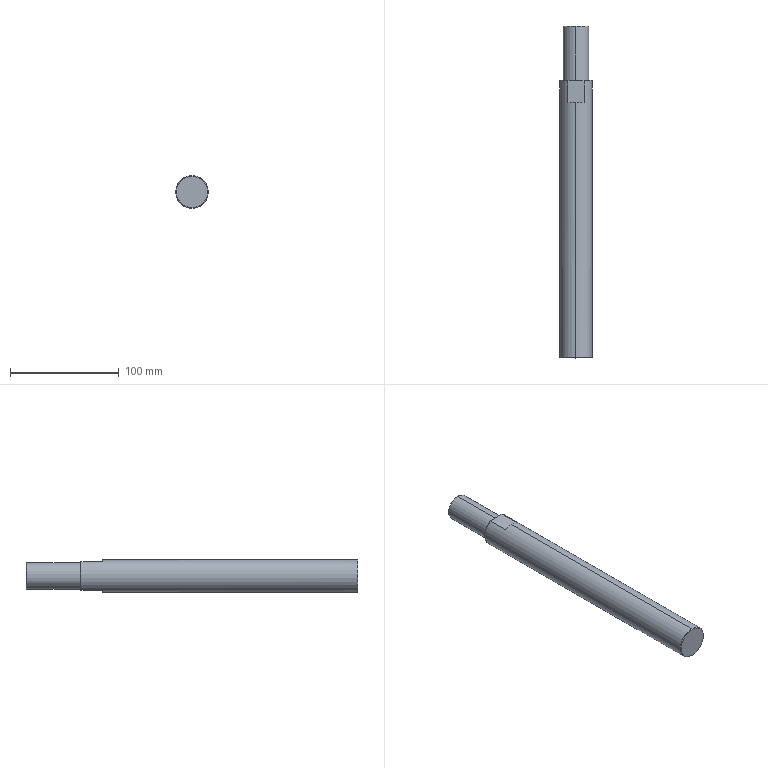Part | STEP file | 30 Plain Shaft | 1 solid | 17 faces | box 30 x 305 x 30 mm | volume 202030 mm3 | plane 7 | cone 6 | cylinder 4 | commonest cylinder face diameters 24 x2 30 x2
STEP:
#1=CARTESIAN_POINT('',(0.,0.,0.));
#2=DIRECTION('',(0.,0.,1.));
#3=DIRECTION('',(1.,0.,0.));
#4=AXIS2_PLACEMENT_3D('',#1,#2,#3);
#5=CARTESIAN_POINT('',(19295.293,8311.493,11.5));
#6=VERTEX_POINT('',#5);
#7=CARTESIAN_POINT('',(19295.293,8311.493,-11.5));
#8=VERTEX_POINT('',#7);
#9=CARTESIAN_POINT('',(19295.293,8311.493,0.));
#10=DIRECTION('',(0.,1.,0.));
#11=DIRECTION('',(0.,0.,1.));
#12=AXIS2_PLACEMENT_3D('',#9,#10,#11);
#13=CIRCLE('',#12,11.5);
#14=CARTESIAN_POINT('',(19295.293,8310.993,0.));
#15=DIRECTION('',(0.,-1.,0.));
#16=DIRECTION('',(0.,0.,-1.));
#17=AXIS2_PLACEMENT_3D('',#14,#15,#16);
#18=CONICAL_SURFACE('',#17,12.,0.7854);
#19=CARTESIAN_POINT('',(3.142,-0.5));
#20=DIRECTION('',(-1.,0.));
#21=VECTOR('',#20,1.);
#22=LINE('',#19,#21);
#23=(GEOMETRIC_REPRESENTATION_CONTEXT(2)PARAMETRIC_REPRESENTATION_CONTEXT()REPRESENTATION_CONTEXT('',''));
#24=DEFINITIONAL_REPRESENTATION('',(#22),#23);
#25=PCURVE('',#18,#24);
#26=CARTESIAN_POINT('',(19306.793,8311.493,0.));
#27=DIRECTION('',(0.,-1.,0.));
#28=DIRECTION('',(0.,0.,-1.));
#29=AXIS2_PLACEMENT_3D('',#26,#27,#28);
#30=PLANE('',#29);
#31=CARTESIAN_POINT('',(-11.5,-11.5));
#32=CARTESIAN_POINT('',(-11.5,8.419));
#33=CARTESIAN_POINT('',(5.75,-1.541));
#34=CARTESIAN_POINT('',(23.,-11.5));
#35=CARTESIAN_POINT('',(5.75,-21.459));
#36=CARTESIAN_POINT('',(-11.5,-31.419));
#37=CARTESIAN_POINT('',(-11.5,-11.5));
#38=(BOUNDED_CURVE()B_SPLINE_CURVE(2,(#31,#32,#33,#34,#35,#36,#37),.UNSPECIFIED.,.T.,.F.)B_SPLINE_CURVE_WITH_KNOTS((1,2,2,2,2,1),(-2.094,0.,2.094,4.189,6.283,8.378),.UNSPECIFIED.)CURVE()GEOMETRIC_REPRESENTATION_ITEM()RATIONAL_B_SPLINE_CURVE((1.,0.5,1.,0.5,1.,0.5,1.))REPRESENTATION_ITEM(''));
#39=(GEOMETRIC_REPRESENTATION_CONTEXT(2)PARAMETRIC_REPRESENTATION_CONTEXT()REPRESENTATION_CONTEXT('',''));
#40=DEFINITIONAL_REPRESENTATION('',(#38),#39);
#41=PCURVE('',#30,#40);
#42=SURFACE_CURVE('',#13,(#25,#41),.PCURVE_S1.);
#43=EDGE_CURVE('',#6,#8,#42,.T.);
#44=ORIENTED_EDGE('',*,*,#43,.F.);
#45=CARTESIAN_POINT('',(19295.293,8310.993,12.));
#46=VERTEX_POINT('',#45);
#47=CARTESIAN_POINT('',(19295.293,8310.993,12.));
#48=DIRECTION('',(0.,-0.7071,0.7071));
#49=VECTOR('',#48,1.);
#50=LINE('',#47,#49);
#51=CARTESIAN_POINT('',(3.142,0.));
#52=DIRECTION('',(0.,1.));
#53=VECTOR('',#52,1.);
#54=LINE('',#51,#53);
#55=(GEOMETRIC_REPRESENTATION_CONTEXT(2)PARAMETRIC_REPRESENTATION_CONTEXT()REPRESENTATION_CONTEXT('',''));
#56=DEFINITIONAL_REPRESENTATION('',(#54),#55);
#57=PCURVE('',#18,#56);
#58=CARTESIAN_POINT('',(19295.293,8310.993,0.));
#59=DIRECTION('',(0.,-1.,0.));
#60=DIRECTION('',(0.,0.,-1.));
#61=AXIS2_PLACEMENT_3D('',#58,#59,#60);
#62=CONICAL_SURFACE('',#61,12.,0.7854);
#63=CARTESIAN_POINT('',(3.142,0.));
#64=DIRECTION('',(0.,1.));
#65=VECTOR('',#64,1.);
#66=LINE('',#63,#65);
#67=(GEOMETRIC_REPRESENTATION_CONTEXT(2)PARAMETRIC_REPRESENTATION_CONTEXT()REPRESENTATION_CONTEXT('',''));
#68=DEFINITIONAL_REPRESENTATION('',(#66),#67);
#69=PCURVE('',#62,#68);
#70=SURFACE_CURVE('',#50,(#57,#69),.PCURVE_S1.);
#71=EDGE_CURVE('',#6,#46,#70,.T.);
#72=ORIENTED_EDGE('',*,*,#71,.T.);
#73=CARTESIAN_POINT('',(19295.293,8310.993,-12.));
#74=VERTEX_POINT('',#73);
#75=CARTESIAN_POINT('',(19295.293,8310.993,0.));
#76=DIRECTION('',(0.,1.,0.));
#77=DIRECTION('',(0.,0.,1.));
#78=AXIS2_PLACEMENT_3D('',#75,#76,#77);
#79=CIRCLE('',#78,12.);
#80=CARTESIAN_POINT('',(3.142,0.));
#81=DIRECTION('',(-1.,0.));
#82=VECTOR('',#81,1.);
#83=LINE('',#80,#82);
#84=(GEOMETRIC_REPRESENTATION_CONTEXT(2)PARAMETRIC_REPRESENTATION_CONTEXT()REPRESENTATION_CONTEXT('',''));
#85=DEFINITIONAL_REPRESENTATION('',(#83),#84);
#86=PCURVE('',#18,#85);
#87=CARTESIAN_POINT('',(19295.293,8358.766,0.));
#88=DIRECTION('',(0.,1.,0.));
#89=DIRECTION('',(0.,0.,1.));
#90=AXIS2_PLACEMENT_3D('',#87,#88,#89);
#91=CYLINDRICAL_SURFACE('',#90,12.);
#92=CARTESIAN_POINT('',(0.,-47.774));
#93=DIRECTION('',(1.,0.));
#94=VECTOR('',#93,1.);
#95=LINE('',#92,#94);
#96=(GEOMETRIC_REPRESENTATION_CONTEXT(2)PARAMETRIC_REPRESENTATION_CONTEXT()REPRESENTATION_CONTEXT('',''));
#97=DEFINITIONAL_REPRESENTATION('',(#95),#96);
#98=PCURVE('',#91,#97);
#99=SURFACE_CURVE('',#79,(#86,#98),.PCURVE_S1.);
#100=EDGE_CURVE('',#46,#74,#99,.T.);
#101=ORIENTED_EDGE('',*,*,#100,.T.);
#102=CARTESIAN_POINT('',(19295.293,8310.993,-12.));
#103=DIRECTION('',(0.,-0.7071,-0.7071));
#104=VECTOR('',#103,1.);
#105=LINE('',#102,#104);
#106=CARTESIAN_POINT('',(0.,0.));
#107=DIRECTION('',(0.,1.));
#108=VECTOR('',#107,1.);
#109=LINE('',#106,#108);
#110=(GEOMETRIC_REPRESENTATION_CONTEXT(2)PARAMETRIC_REPRESENTATION_CONTEXT()REPRESENTATION_CONTEXT('',''));
#111=DEFINITIONAL_REPRESENTATION('',(#109),#110);
#112=PCURVE('',#18,#111);
#113=CARTESIAN_POINT('',(6.283,0.));
#114=DIRECTION('',(0.,1.));
#115=VECTOR('',#114,1.);
#116=LINE('',#113,#115);
#117=(GEOMETRIC_REPRESENTATION_CONTEXT(2)PARAMETRIC_REPRESENTATION_CONTEXT()REPRESENTATION_CONTEXT('',''));
#118=DEFINITIONAL_REPRESENTATION('',(#116),#117);
#119=PCURVE('',#62,#118);
#120=SURFACE_CURVE('',#105,(#112,#119),.PCURVE_S1.);
#121=EDGE_CURVE('',#8,#74,#120,.T.);
#122=ORIENTED_EDGE('',*,*,#121,.F.);
#123=EDGE_LOOP('',(#44,#72,#101,#122));
#124=FACE_BOUND('',#123,.T.);
#125=ADVANCED_FACE('',(#124),#18,.T.);
#126=CARTESIAN_POINT('',(19295.293,8261.493,12.));
#127=VERTEX_POINT('',#126);
#128=CARTESIAN_POINT('',(19295.293,8261.493,-12.));
#129=VERTEX_POINT('',#128);
#130=CARTESIAN_POINT('',(19295.293,8261.493,0.));
#131=DIRECTION('',(0.,1.,0.));
#132=DIRECTION('',(0.,0.,1.));
#133=AXIS2_PLACEMENT_3D('',#130,#131,#132);
#134=CIRCLE('',#133,12.);
#135=CARTESIAN_POINT('',(0.,-97.274));
#136=DIRECTION('',(1.,0.));
#137=VECTOR('',#136,1.);
#138=LINE('',#135,#137);
#139=(GEOMETRIC_REPRESENTATION_CONTEXT(2)PARAMETRIC_REPRESENTATION_CONTEXT()REPRESENTATION_CONTEXT('',''));
#140=DEFINITIONAL_REPRESENTATION('',(#138),#139);
#141=PCURVE('',#91,#140);
#142=CARTESIAN_POINT('',(19309.793,8261.493,0.));
#143=DIRECTION('',(0.,-1.,0.));
#144=DIRECTION('',(0.,0.,-1.));
#145=AXIS2_PLACEMENT_3D('',#142,#143,#144);
#146=PLANE('',#145);
#147=CARTESIAN_POINT('',(-12.,-14.5));
#148=CARTESIAN_POINT('',(-12.,6.285));
#149=CARTESIAN_POINT('',(6.,-4.108));
#150=CARTESIAN_POINT('',(24.,-14.5));
#151=CARTESIAN_POINT('',(6.,-24.892));
#152=CARTESIAN_POINT('',(-12.,-35.285));
#153=CARTESIAN_POINT('',(-12.,-14.5));
#154=(BOUNDED_CURVE()B_SPLINE_CURVE(2,(#147,#148,#149,#150,#151,#152,#153),.UNSPECIFIED.,.T.,.F.)B_SPLINE_CURVE_WITH_KNOTS((1,2,2,2,2,1),(-2.094,0.,2.094,4.189,6.283,8.378),.UNSPECIFIED.)CURVE()GEOMETRIC_REPRESENTATION_ITEM()RATIONAL_B_SPLINE_CURVE((1.,0.5,1.,0.5,1.,0.5,1.))REPRESENTATION_ITEM(''));
#155=(GEOMETRIC_REPRESENTATION_CONTEXT(2)PARAMETRIC_REPRESENTATION_CONTEXT()REPRESENTATION_CONTEXT('',''));
#156=DEFINITIONAL_REPRESENTATION('',(#154),#155);
#157=PCURVE('',#146,#156);
#158=SURFACE_CURVE('',#134,(#141,#157),.PCURVE_S1.);
#159=EDGE_CURVE('',#127,#129,#158,.T.);
#160=ORIENTED_EDGE('',*,*,#159,.T.);
#161=CARTESIAN_POINT('',(19295.293,8358.766,-12.));
#162=DIRECTION('',(0.,1.,0.));
#163=VECTOR('',#162,1.);
#164=LINE('',#161,#163);
#165=CARTESIAN_POINT('',(3.142,0.));
#166=DIRECTION('',(0.,1.));
#167=VECTOR('',#166,1.);
#168=LINE('',#165,#167);
#169=(GEOMETRIC_REPRESENTATION_CONTEXT(2)PARAMETRIC_REPRESENTATION_CONTEXT()REPRESENTATION_CONTEXT('',''));
#170=DEFINITIONAL_REPRESENTATION('',(#168),#169);
#171=PCURVE('',#91,#170);
#172=CARTESIAN_POINT('',(19295.293,8358.766,0.));
#173=DIRECTION('',(0.,1.,0.));
#174=DIRECTION('',(0.,0.,1.));
#175=AXIS2_PLACEMENT_3D('',#172,#173,#174);
#176=CYLINDRICAL_SURFACE('',#175,12.);
#177=CARTESIAN_POINT('',(3.142,0.));
#178=DIRECTION('',(0.,1.));
#179=VECTOR('',#178,1.);
#180=LINE('',#177,#179);
#181=(GEOMETRIC_REPRESENTATION_CONTEXT(2)PARAMETRIC_REPRESENTATION_CONTEXT()REPRESENTATION_CONTEXT('',''));
#182=DEFINITIONAL_REPRESENTATION('',(#180),#181);
#183=PCURVE('',#176,#182);
#184=SURFACE_CURVE('',#164,(#171,#183),.PCURVE_S1.);
#185=EDGE_CURVE('',#129,#74,#184,.T.);
#186=ORIENTED_EDGE('',*,*,#185,.T.);
#187=ORIENTED_EDGE('',*,*,#100,.F.);
#188=CARTESIAN_POINT('',(19295.293,8358.766,12.));
#189=DIRECTION('',(0.,1.,0.));
#190=VECTOR('',#189,1.);
#191=LINE('',#188,#190);
#192=CARTESIAN_POINT('',(0.,0.));
#193=DIRECTION('',(0.,1.));
#194=VECTOR('',#193,1.);
#195=LINE('',#192,#194);
#196=(GEOMETRIC_REPRESENTATION_CONTEXT(2)PARAMETRIC_REPRESENTATION_CONTEXT()REPRESENTATION_CONTEXT('',''));
#197=DEFINITIONAL_REPRESENTATION('',(#195),#196);
#198=PCURVE('',#91,#197);
#199=CARTESIAN_POINT('',(6.283,0.));
#200=DIRECTION('',(0.,1.));
#201=VECTOR('',#200,1.);
#202=LINE('',#199,#201);
#203=(GEOMETRIC_REPRESENTATION_CONTEXT(2)PARAMETRIC_REPRESENTATION_CONTEXT()REPRESENTATION_CONTEXT('',''));
#204=DEFINITIONAL_REPRESENTATION('',(#202),#203);
#205=PCURVE('',#176,#204);
#206=SURFACE_CURVE('',#191,(#198,#205),.PCURVE_S1.);
#207=EDGE_CURVE('',#127,#46,#206,.T.);
#208=ORIENTED_EDGE('',*,*,#207,.F.);
#209=EDGE_LOOP('',(#160,#186,#187,#208));
#210=FACE_BOUND('',#209,.T.);
#211=ADVANCED_FACE('',(#210),#91,.T.);
#212=CARTESIAN_POINT('',(19295.293,8006.993,15.));
#213=VERTEX_POINT('',#212);
#214=CARTESIAN_POINT('',(19295.293,8006.993,-15.));
#215=VERTEX_POINT('',#214);
#216=CARTESIAN_POINT('',(19295.293,8006.993,0.));
#217=DIRECTION('',(0.,1.,0.));
#218=DIRECTION('',(0.,0.,1.));
#219=AXIS2_PLACEMENT_3D('',#216,#217,#218);
#220=CIRCLE('',#219,15.);
#221=CARTESIAN_POINT('',(19295.293,8358.766,0.));
#222=DIRECTION('',(0.,1.,0.));
#223=DIRECTION('',(0.,0.,1.));
#224=AXIS2_PLACEMENT_3D('',#221,#222,#223);
#225=CYLINDRICAL_SURFACE('',#224,15.);
#226=CARTESIAN_POINT('',(0.,-351.774));
#227=DIRECTION('',(1.,0.));
#228=VECTOR('',#227,1.);
#229=LINE('',#226,#228);
#230=(GEOMETRIC_REPRESENTATION_CONTEXT(2)PARAMETRIC_REPRESENTATION_CONTEXT()REPRESENTATION_CONTEXT('',''));
#231=DEFINITIONAL_REPRESENTATION('',(#229),#230);
#232=PCURVE('',#225,#231);
#233=CARTESIAN_POINT('',(19295.293,8006.493,0.));
#234=DIRECTION('',(0.,1.,0.));
#235=DIRECTION('',(0.,0.,1.));
#236=AXIS2_PLACEMENT_3D('',#233,#234,#235);
#237=CONICAL_SURFACE('',#236,14.5,0.7854);
#238=CARTESIAN_POINT('',(0.,0.5));
#239=DIRECTION('',(1.,0.));
#240=VECTOR('',#239,1.);
#241=LINE('',#238,#240);
#242=(GEOMETRIC_REPRESENTATION_CONTEXT(2)PARAMETRIC_REPRESENTATION_CONTEXT()REPRESENTATION_CONTEXT('',''));
#243=DEFINITIONAL_REPRESENTATION('',(#241),#242);
#244=PCURVE('',#237,#243);
#245=SURFACE_CURVE('',#220,(#232,#244),.PCURVE_S1.);
#246=EDGE_CURVE('',#213,#215,#245,.T.);
#247=ORIENTED_EDGE('',*,*,#246,.T.);
#248=CARTESIAN_POINT('',(19295.293,8241.493,-15.));
#249=VERTEX_POINT('',#248);
#250=CARTESIAN_POINT('',(19295.293,8358.766,-15.));
#251=DIRECTION('',(0.,1.,0.));
#252=VECTOR('',#251,1.);
#253=LINE('',#250,#252);
#254=CARTESIAN_POINT('',(3.142,0.));
#255=DIRECTION('',(0.,1.));
#256=VECTOR('',#255,1.);
#257=LINE('',#254,#256);
#258=(GEOMETRIC_REPRESENTATION_CONTEXT(2)PARAMETRIC_REPRESENTATION_CONTEXT()REPRESENTATION_CONTEXT('',''));
#259=DEFINITIONAL_REPRESENTATION('',(#257),#258);
#260=PCURVE('',#225,#259);
#261=CARTESIAN_POINT('',(19295.293,8358.766,0.));
#262=DIRECTION('',(0.,1.,0.));
#263=DIRECTION('',(0.,0.,1.));
#264=AXIS2_PLACEMENT_3D('',#261,#262,#263);
#265=CYLINDRICAL_SURFACE('',#264,15.);
#266=CARTESIAN_POINT('',(3.142,0.));
#267=DIRECTION('',(0.,1.));
#268=VECTOR('',#267,1.);
#269=LINE('',#266,#268);
#270=(GEOMETRIC_REPRESENTATION_CONTEXT(2)PARAMETRIC_REPRESENTATION_CONTEXT()REPRESENTATION_CONTEXT('',''));
#271=DEFINITIONAL_REPRESENTATION('',(#269),#270);
#272=PCURVE('',#265,#271);
#273=SURFACE_CURVE('',#253,(#260,#272),.PCURVE_S1.);
#274=EDGE_CURVE('',#215,#249,#273,.T.);
#275=ORIENTED_EDGE('',*,*,#274,.T.);
#276=CARTESIAN_POINT('',(19302.777,8241.493,-13.));
#277=VERTEX_POINT('',#276);
#278=CARTESIAN_POINT('',(19295.293,8241.493,0.));
#279=DIRECTION('',(0.,1.,0.));
#280=DIRECTION('',(0.,0.,1.));
#281=AXIS2_PLACEMENT_3D('',#278,#279,#280);
#282=CIRCLE('',#281,15.);
#283=CARTESIAN_POINT('',(0.,-117.274));
#284=DIRECTION('',(1.,0.));
#285=VECTOR('',#284,1.);
#286=LINE('',#283,#285);
#287=(GEOMETRIC_REPRESENTATION_CONTEXT(2)PARAMETRIC_REPRESENTATION_CONTEXT()REPRESENTATION_CONTEXT('',''));
#288=DEFINITIONAL_REPRESENTATION('',(#286),#287);
#289=PCURVE('',#225,#288);
#290=CARTESIAN_POINT('',(0.,8241.493,0.));
#291=DIRECTION('',(0.,1.,0.));
#292=DIRECTION('',(0.,0.,1.));
#293=AXIS2_PLACEMENT_3D('',#290,#291,#292);
#294=PLANE('',#293);
#295=CARTESIAN_POINT('',(0.,19295.293));
#296=DIRECTION('',(1.,0.));
#297=AXIS2_PLACEMENT_2D('',#295,#296);
#298=CIRCLE('',#297,15.);
#299=(GEOMETRIC_REPRESENTATION_CONTEXT(2)PARAMETRIC_REPRESENTATION_CONTEXT()REPRESENTATION_CONTEXT('',''));
#300=DEFINITIONAL_REPRESENTATION('',(#298),#299);
#301=PCURVE('',#294,#300);
#302=SURFACE_CURVE('',#282,(#289,#301),.PCURVE_S1.);
#303=EDGE_CURVE('',#277,#249,#302,.T.);
#304=ORIENTED_EDGE('',*,*,#303,.F.);
#305=CARTESIAN_POINT('',(19302.777,8260.993,-13.));
#306=VERTEX_POINT('',#305);
#307=CARTESIAN_POINT('',(19302.777,8358.766,-13.));
#308=DIRECTION('',(0.,1.,0.));
#309=VECTOR('',#308,1.);
#310=LINE('',#307,#309);
#311=CARTESIAN_POINT('',(2.619,0.));
#312=DIRECTION('',(0.,1.));
#313=VECTOR('',#312,1.);
#314=LINE('',#311,#313);
#315=(GEOMETRIC_REPRESENTATION_CONTEXT(2)PARAMETRIC_REPRESENTATION_CONTEXT()REPRESENTATION_CONTEXT('',''));
#316=DEFINITIONAL_REPRESENTATION('',(#314),#315);
#317=PCURVE('',#225,#316);
#318=CARTESIAN_POINT('',(19265.494,8241.493,-13.));
#319=DIRECTION('',(0.,0.,1.));
#320=DIRECTION('',(1.,0.,0.));
#321=AXIS2_PLACEMENT_3D('',#318,#319,#320);
#322=PLANE('',#321);
#323=CARTESIAN_POINT('',(37.282,117.274));
#324=DIRECTION('',(0.,1.));
#325=VECTOR('',#324,1.);
#326=LINE('',#323,#325);
#327=(GEOMETRIC_REPRESENTATION_CONTEXT(2)PARAMETRIC_REPRESENTATION_CONTEXT()REPRESENTATION_CONTEXT('',''));
#328=DEFINITIONAL_REPRESENTATION('',(#326),#327);
#329=PCURVE('',#322,#328);
#330=SURFACE_CURVE('',#310,(#317,#329),.PCURVE_S1.);
#331=EDGE_CURVE('',#277,#306,#330,.T.);
#332=ORIENTED_EDGE('',*,*,#331,.T.);
#333=CARTESIAN_POINT('',(19302.777,8260.993,13.));
#334=VERTEX_POINT('',#333);
#335=CARTESIAN_POINT('',(19295.293,8260.993,0.));
#336=DIRECTION('',(0.,1.,0.));
#337=DIRECTION('',(0.,0.,1.));
#338=AXIS2_PLACEMENT_3D('',#335,#336,#337);
#339=CIRCLE('',#338,15.);
#340=CARTESIAN_POINT('',(0.,-97.774));
#341=DIRECTION('',(1.,0.));
#342=VECTOR('',#341,1.);
#343=LINE('',#340,#342);
#344=(GEOMETRIC_REPRESENTATION_CONTEXT(2)PARAMETRIC_REPRESENTATION_CONTEXT()REPRESENTATION_CONTEXT('',''));
#345=DEFINITIONAL_REPRESENTATION('',(#343),#344);
#346=PCURVE('',#225,#345);
#347=CARTESIAN_POINT('',(19295.293,8260.993,0.));
#348=DIRECTION('',(0.,-1.,0.));
#349=DIRECTION('',(0.,0.,-1.));
#350=AXIS2_PLACEMENT_3D('',#347,#348,#349);
#351=CONICAL_SURFACE('',#350,15.,0.7854);
#352=CARTESIAN_POINT('',(3.142,0.));
#353=DIRECTION('',(-1.,0.));
#354=VECTOR('',#353,1.);
#355=LINE('',#352,#354);
#356=(GEOMETRIC_REPRESENTATION_CONTEXT(2)PARAMETRIC_REPRESENTATION_CONTEXT()REPRESENTATION_CONTEXT('',''));
#357=DEFINITIONAL_REPRESENTATION('',(#355),#356);
#358=PCURVE('',#351,#357);
#359=SURFACE_CURVE('',#339,(#346,#358),.PCURVE_S1.);
#360=EDGE_CURVE('',#334,#306,#359,.T.);
#361=ORIENTED_EDGE('',*,*,#360,.F.);
#362=CARTESIAN_POINT('',(19302.777,8241.493,13.));
#363=VERTEX_POINT('',#362);
#364=CARTESIAN_POINT('',(19302.777,8358.766,13.));
#365=DIRECTION('',(0.,-1.,0.));
#366=VECTOR('',#365,1.);
#367=LINE('',#364,#366);
#368=CARTESIAN_POINT('',(0.5223,0.));
#369=DIRECTION('',(0.,-1.));
#370=VECTOR('',#369,1.);
#371=LINE('',#368,#370);
#372=(GEOMETRIC_REPRESENTATION_CONTEXT(2)PARAMETRIC_REPRESENTATION_CONTEXT()REPRESENTATION_CONTEXT('',''));
#373=DEFINITIONAL_REPRESENTATION('',(#371),#372);
#374=PCURVE('',#225,#373);
#375=CARTESIAN_POINT('',(19286.893,8241.493,13.));
#376=DIRECTION('',(0.,0.,-1.));
#377=DIRECTION('',(-1.,0.,0.));
#378=AXIS2_PLACEMENT_3D('',#375,#376,#377);
#379=PLANE('',#378);
#380=CARTESIAN_POINT('',(-15.884,117.274));
#381=DIRECTION('',(0.,-1.));
#382=VECTOR('',#381,1.);
#383=LINE('',#380,#382);
#384=(GEOMETRIC_REPRESENTATION_CONTEXT(2)PARAMETRIC_REPRESENTATION_CONTEXT()REPRESENTATION_CONTEXT('',''));
#385=DEFINITIONAL_REPRESENTATION('',(#383),#384);
#386=PCURVE('',#379,#385);
#387=SURFACE_CURVE('',#367,(#374,#386),.PCURVE_S1.);
#388=EDGE_CURVE('',#334,#363,#387,.T.);
#389=ORIENTED_EDGE('',*,*,#388,.T.);
#390=CARTESIAN_POINT('',(19295.293,8241.493,15.));
#391=VERTEX_POINT('',#390);
#392=CARTESIAN_POINT('',(19295.293,8241.493,0.));
#393=DIRECTION('',(0.,-1.,0.));
#394=DIRECTION('',(0.,0.,-1.));
#395=AXIS2_PLACEMENT_3D('',#392,#393,#394);
#396=CIRCLE('',#395,15.);
#397=CARTESIAN_POINT('',(3.142,-117.274));
#398=DIRECTION('',(-1.,0.));
#399=VECTOR('',#398,1.);
#400=LINE('',#397,#399);
#401=(GEOMETRIC_REPRESENTATION_CONTEXT(2)PARAMETRIC_REPRESENTATION_CONTEXT()REPRESENTATION_CONTEXT('',''));
#402=DEFINITIONAL_REPRESENTATION('',(#400),#401);
#403=PCURVE('',#225,#402);
#404=CARTESIAN_POINT('',(0.,8241.493,0.));
#405=DIRECTION('',(0.,-1.,0.));
#406=DIRECTION('',(0.,0.,-1.));
#407=AXIS2_PLACEMENT_3D('',#404,#405,#406);
#408=PLANE('',#407);
#409=CARTESIAN_POINT('',(0.,19295.293));
#410=DIRECTION('',(1.,0.));
#411=AXIS2_PLACEMENT_2D('',#409,#410);
#412=CIRCLE('',#411,15.);
#413=(GEOMETRIC_REPRESENTATION_CONTEXT(2)PARAMETRIC_REPRESENTATION_CONTEXT()REPRESENTATION_CONTEXT('',''));
#414=DEFINITIONAL_REPRESENTATION('',(#412),#413);
#415=PCURVE('',#408,#414);
#416=SURFACE_CURVE('',#396,(#403,#415),.PCURVE_S1.);
#417=EDGE_CURVE('',#363,#391,#416,.T.);
#418=ORIENTED_EDGE('',*,*,#417,.T.);
#419=CARTESIAN_POINT('',(19295.293,8358.766,15.));
#420=DIRECTION('',(0.,1.,0.));
#421=VECTOR('',#420,1.);
#422=LINE('',#419,#421);
#423=CARTESIAN_POINT('',(0.,0.));
#424=DIRECTION('',(0.,1.));
#425=VECTOR('',#424,1.);
#426=LINE('',#423,#425);
#427=(GEOMETRIC_REPRESENTATION_CONTEXT(2)PARAMETRIC_REPRESENTATION_CONTEXT()REPRESENTATION_CONTEXT('',''));
#428=DEFINITIONAL_REPRESENTATION('',(#426),#427);
#429=PCURVE('',#225,#428);
#430=CARTESIAN_POINT('',(6.283,0.));
#431=DIRECTION('',(0.,1.));
#432=VECTOR('',#431,1.);
#433=LINE('',#430,#432);
#434=(GEOMETRIC_REPRESENTATION_CONTEXT(2)PARAMETRIC_REPRESENTATION_CONTEXT()REPRESENTATION_CONTEXT('',''));
#435=DEFINITIONAL_REPRESENTATION('',(#433),#434);
#436=PCURVE('',#265,#435);
#437=SURFACE_CURVE('',#422,(#429,#436),.PCURVE_S1.);
#438=EDGE_CURVE('',#213,#391,#437,.T.);
#439=ORIENTED_EDGE('',*,*,#438,.F.);
#440=EDGE_LOOP('',(#247,#275,#304,#332,#361,#389,#418,#439));
#441=FACE_BOUND('',#440,.T.);
#442=ADVANCED_FACE('',(#441),#225,.T.);
#443=CARTESIAN_POINT('',(19295.293,8006.493,14.5));
#444=VERTEX_POINT('',#443);
#445=CARTESIAN_POINT('',(19295.293,8006.493,-14.5));
#446=VERTEX_POINT('',#445);
#447=CARTESIAN_POINT('',(19295.293,8006.493,0.));
#448=DIRECTION('',(0.,1.,0.));
#449=DIRECTION('',(0.,0.,1.));
#450=AXIS2_PLACEMENT_3D('',#447,#448,#449);
#451=CIRCLE('',#450,14.5);
#452=CARTESIAN_POINT('',(0.,0.));
#453=DIRECTION('',(1.,0.));
#454=VECTOR('',#453,1.);
#455=LINE('',#452,#454);
#456=(GEOMETRIC_REPRESENTATION_CONTEXT(2)PARAMETRIC_REPRESENTATION_CONTEXT()REPRESENTATION_CONTEXT('',''));
#457=DEFINITIONAL_REPRESENTATION('',(#455),#456);
#458=PCURVE('',#237,#457);
#459=CARTESIAN_POINT('',(19307.293,8006.493,0.));
#460=DIRECTION('',(0.,1.,0.));
#461=DIRECTION('',(0.,0.,1.));
#462=AXIS2_PLACEMENT_3D('',#459,#460,#461);
#463=PLANE('',#462);
#464=CARTESIAN_POINT('',(0.,-12.));
#465=DIRECTION('',(1.,0.));
#466=AXIS2_PLACEMENT_2D('',#464,#465);
#467=CIRCLE('',#466,14.5);
#468=(GEOMETRIC_REPRESENTATION_CONTEXT(2)PARAMETRIC_REPRESENTATION_CONTEXT()REPRESENTATION_CONTEXT('',''));
#469=DEFINITIONAL_REPRESENTATION('',(#467),#468);
#470=PCURVE('',#463,#469);
#471=SURFACE_CURVE('',#451,(#458,#470),.PCURVE_S1.);
#472=EDGE_CURVE('',#444,#446,#471,.T.);
#473=ORIENTED_EDGE('',*,*,#472,.T.);
#474=CARTESIAN_POINT('',(19295.293,8006.493,-14.5));
#475=DIRECTION('',(0.,0.7071,-0.7071));
#476=VECTOR('',#475,1.);
#477=LINE('',#474,#476);
#478=CARTESIAN_POINT('',(3.142,0.));
#479=DIRECTION('',(0.,1.));
#480=VECTOR('',#479,1.);
#481=LINE('',#478,#480);
#482=(GEOMETRIC_REPRESENTATION_CONTEXT(2)PARAMETRIC_REPRESENTATION_CONTEXT()REPRESENTATION_CONTEXT('',''));
#483=DEFINITIONAL_REPRESENTATION('',(#481),#482);
#484=PCURVE('',#237,#483);
#485=CARTESIAN_POINT('',(19295.293,8006.493,0.));
#486=DIRECTION('',(0.,1.,0.));
#487=DIRECTION('',(0.,0.,1.));
#488=AXIS2_PLACEMENT_3D('',#485,#486,#487);
#489=CONICAL_SURFACE('',#488,14.5,0.7854);
#490=CARTESIAN_POINT('',(3.142,0.));
#491=DIRECTION('',(0.,1.));
#492=VECTOR('',#491,1.);
#493=LINE('',#490,#492);
#494=(GEOMETRIC_REPRESENTATION_CONTEXT(2)PARAMETRIC_REPRESENTATION_CONTEXT()REPRESENTATION_CONTEXT('',''));
#495=DEFINITIONAL_REPRESENTATION('',(#493),#494);
#496=PCURVE('',#489,#495);
#497=SURFACE_CURVE('',#477,(#484,#496),.PCURVE_S1.);
#498=EDGE_CURVE('',#446,#215,#497,.T.);
#499=ORIENTED_EDGE('',*,*,#498,.T.);
#500=ORIENTED_EDGE('',*,*,#246,.F.);
#501=CARTESIAN_POINT('',(19295.293,8006.493,14.5));
#502=DIRECTION('',(0.,0.7071,0.7071));
#503=VECTOR('',#502,1.);
#504=LINE('',#501,#503);
#505=CARTESIAN_POINT('',(0.,0.));
#506=DIRECTION('',(0.,1.));
#507=VECTOR('',#506,1.);
#508=LINE('',#505,#507);
#509=(GEOMETRIC_REPRESENTATION_CONTEXT(2)PARAMETRIC_REPRESENTATION_CONTEXT()REPRESENTATION_CONTEXT('',''));
#510=DEFINITIONAL_REPRESENTATION('',(#508),#509);
#511=PCURVE('',#237,#510);
#512=CARTESIAN_POINT('',(6.283,0.));
#513=DIRECTION('',(0.,1.));
#514=VECTOR('',#513,1.);
#515=LINE('',#512,#514);
#516=(GEOMETRIC_REPRESENTATION_CONTEXT(2)PARAMETRIC_REPRESENTATION_CONTEXT()REPRESENTATION_CONTEXT('',''));
#517=DEFINITIONAL_REPRESENTATION('',(#515),#516);
#518=PCURVE('',#489,#517);
#519=SURFACE_CURVE('',#504,(#511,#518),.PCURVE_S1.);
#520=EDGE_CURVE('',#444,#213,#519,.T.);
#521=ORIENTED_EDGE('',*,*,#520,.F.);
#522=EDGE_LOOP('',(#473,#499,#500,#521));
#523=FACE_BOUND('',#522,.T.);
#524=ADVANCED_FACE('',(#523),#237,.T.);
#525=CARTESIAN_POINT('',(19287.81,8260.993,-13.));
#526=VERTEX_POINT('',#525);
#527=CARTESIAN_POINT('',(19287.81,8260.993,13.));
#528=VERTEX_POINT('',#527);
#529=CARTESIAN_POINT('',(19295.293,8260.993,0.));
#530=DIRECTION('',(0.,1.,0.));
#531=DIRECTION('',(0.,0.,1.));
#532=AXIS2_PLACEMENT_3D('',#529,#530,#531);
#533=CIRCLE('',#532,15.);
#534=CARTESIAN_POINT('',(19295.293,8260.993,0.));
#535=DIRECTION('',(0.,-1.,0.));
#536=DIRECTION('',(0.,0.,-1.));
#537=AXIS2_PLACEMENT_3D('',#534,#535,#536);
#538=CONICAL_SURFACE('',#537,15.,0.7854);
#539=CARTESIAN_POINT('',(9.425,0.));
#540=DIRECTION('',(-1.,0.));
#541=VECTOR('',#540,1.);
#542=LINE('',#539,#541);
#543=(GEOMETRIC_REPRESENTATION_CONTEXT(2)PARAMETRIC_REPRESENTATION_CONTEXT()REPRESENTATION_CONTEXT('',''));
#544=DEFINITIONAL_REPRESENTATION('',(#542),#543);
#545=PCURVE('',#538,#544);
#546=CARTESIAN_POINT('',(0.,-97.774));
#547=DIRECTION('',(1.,0.));
#548=VECTOR('',#547,1.);
#549=LINE('',#546,#548);
#550=(GEOMETRIC_REPRESENTATION_CONTEXT(2)PARAMETRIC_REPRESENTATION_CONTEXT()REPRESENTATION_CONTEXT('',''));
#551=DEFINITIONAL_REPRESENTATION('',(#549),#550);
#552=PCURVE('',#265,#551);
#553=SURFACE_CURVE('',#533,(#545,#552),.PCURVE_S1.);
#554=EDGE_CURVE('',#526,#528,#553,.T.);
#555=ORIENTED_EDGE('',*,*,#554,.T.);
#556=CARTESIAN_POINT('',(19288.871,8261.493,13.));
#557=VERTEX_POINT('',#556);
#558=CARTESIAN_POINT('',(19287.81,8260.993,13.));
#559=CARTESIAN_POINT('',(19288.159,8261.167,13.));
#560=CARTESIAN_POINT('',(19288.512,8261.334,13.));
#561=CARTESIAN_POINT('',(19288.871,8261.493,13.));
#562=B_SPLINE_CURVE_WITH_KNOTS('',3,(#558,#559,#560,#561),.UNSPECIFIED.,.F.,.F.,(4,4),(0.0186,0.01977),.PIECEWISE_BEZIER_KNOTS.);
#563=CARTESIAN_POINT('',(3.664,0.));
#564=CARTESIAN_POINT('',(3.663,-0.007919));
#565=CARTESIAN_POINT('',(3.661,-0.02373));
#566=CARTESIAN_POINT('',(3.658,-0.04735));
#567=CARTESIAN_POINT('',(3.656,-0.07089));
#568=CARTESIAN_POINT('',(3.653,-0.09433));
#569=CARTESIAN_POINT('',(3.65,-0.1177));
#570=CARTESIAN_POINT('',(3.647,-0.141));
#571=CARTESIAN_POINT('',(3.644,-0.1641));
#572=CARTESIAN_POINT('',(3.642,-0.1872));
#573=CARTESIAN_POINT('',(3.639,-0.2102));
#574=CARTESIAN_POINT('',(3.636,-0.2331));
#575=CARTESIAN_POINT('',(3.633,-0.2559));
#576=CARTESIAN_POINT('',(3.63,-0.2786));
#577=CARTESIAN_POINT('',(3.627,-0.3011));
#578=CARTESIAN_POINT('',(3.624,-0.3236));
#579=CARTESIAN_POINT('',(3.621,-0.346));
#580=CARTESIAN_POINT('',(3.618,-0.3683));
#581=CARTESIAN_POINT('',(3.615,-0.3905));
#582=CARTESIAN_POINT('',(3.612,-0.4126));
#583=CARTESIAN_POINT('',(3.609,-0.4346));
#584=CARTESIAN_POINT('',(3.606,-0.4565));
#585=CARTESIAN_POINT('',(3.603,-0.4783));
#586=CARTESIAN_POINT('',(3.601,-0.4928));
#587=CARTESIAN_POINT('',(3.6,-0.5));
#588=B_SPLINE_CURVE_WITH_KNOTS('',3,(#563,#564,#565,#566,#567,#568,#569,#570,#571,#572,#573,#574,#575,#576,#577,#578,#579,#580,#581,#582,#583,#584,#585,#586,#587),.UNSPECIFIED.,.F.,.F.,(4,1,1,1,1,1,1,1,1,1,1,1,1,1,1,1,1,1,1,1,1,1,4),(0.0186,0.01865,0.01871,0.01876,0.01881,0.01887,0.01892,0.01897,0.01903,0.01908,0.01913,0.01919,0.01924,0.01929,0.01935,0.0194,0.01945,0.01951,0.01956,0.01961,0.01967,0.01972,0.01977),.QUASI_UNIFORM_KNOTS.);
#589=(GEOMETRIC_REPRESENTATION_CONTEXT(2)PARAMETRIC_REPRESENTATION_CONTEXT()REPRESENTATION_CONTEXT('',''));
#590=DEFINITIONAL_REPRESENTATION('',(#588),#589);
#591=PCURVE('',#538,#590);
#592=CARTESIAN_POINT('',(-0.917,19.5));
#593=CARTESIAN_POINT('',(-1.266,19.674));
#594=CARTESIAN_POINT('',(-1.62,19.841));
#595=CARTESIAN_POINT('',(-1.978,20.));
#596=B_SPLINE_CURVE_WITH_KNOTS('',3,(#592,#593,#594,#595),.UNSPECIFIED.,.F.,.F.,(4,4),(0.0186,0.01977),.PIECEWISE_BEZIER_KNOTS.);
#597=(GEOMETRIC_REPRESENTATION_CONTEXT(2)PARAMETRIC_REPRESENTATION_CONTEXT()REPRESENTATION_CONTEXT('',''));
#598=DEFINITIONAL_REPRESENTATION('',(#596),#597);
#599=PCURVE('',#379,#598);
#600=SURFACE_CURVE('',#562,(#591,#599),.PCURVE_S1.);
#601=EDGE_CURVE('',#528,#557,#600,.T.);
#602=ORIENTED_EDGE('',*,*,#601,.T.);
#603=CARTESIAN_POINT('',(19288.871,8261.493,-13.));
#604=VERTEX_POINT('',#603);
#605=CARTESIAN_POINT('',(19295.293,8261.493,0.));
#606=DIRECTION('',(0.,1.,0.));
#607=DIRECTION('',(0.,0.,1.));
#608=AXIS2_PLACEMENT_3D('',#605,#606,#607);
#609=CIRCLE('',#608,14.5);
#610=CARTESIAN_POINT('',(9.425,-0.5));
#611=DIRECTION('',(-1.,0.));
#612=VECTOR('',#611,1.);
#613=LINE('',#610,#612);
#614=(GEOMETRIC_REPRESENTATION_CONTEXT(2)PARAMETRIC_REPRESENTATION_CONTEXT()REPRESENTATION_CONTEXT('',''));
#615=DEFINITIONAL_REPRESENTATION('',(#613),#614);
#616=PCURVE('',#538,#615);
#617=CARTESIAN_POINT('',(-14.5,-14.5));
#618=CARTESIAN_POINT('',(-14.5,10.615));
#619=CARTESIAN_POINT('',(7.25,-1.943));
#620=CARTESIAN_POINT('',(29.,-14.5));
#621=CARTESIAN_POINT('',(7.25,-27.057));
#622=CARTESIAN_POINT('',(-14.5,-39.615));
#623=CARTESIAN_POINT('',(-14.5,-14.5));
#624=(BOUNDED_CURVE()B_SPLINE_CURVE(2,(#617,#618,#619,#620,#621,#622,#623),.UNSPECIFIED.,.T.,.F.)B_SPLINE_CURVE_WITH_KNOTS((1,2,2,2,2,1),(-2.094,0.,2.094,4.189,6.283,8.378),.UNSPECIFIED.)CURVE()GEOMETRIC_REPRESENTATION_ITEM()RATIONAL_B_SPLINE_CURVE((1.,0.5,1.,0.5,1.,0.5,1.))REPRESENTATION_ITEM(''));
#625=(GEOMETRIC_REPRESENTATION_CONTEXT(2)PARAMETRIC_REPRESENTATION_CONTEXT()REPRESENTATION_CONTEXT('',''));
#626=DEFINITIONAL_REPRESENTATION('',(#624),#625);
#627=PCURVE('',#146,#626);
#628=SURFACE_CURVE('',#609,(#616,#627),.PCURVE_S1.);
#629=EDGE_CURVE('',#604,#557,#628,.T.);
#630=ORIENTED_EDGE('',*,*,#629,.F.);
#631=CARTESIAN_POINT('',(19288.871,8261.493,-13.));
#632=CARTESIAN_POINT('',(19288.512,8261.334,-13.));
#633=CARTESIAN_POINT('',(19288.159,8261.167,-13.));
#634=CARTESIAN_POINT('',(19287.81,8260.993,-13.));
#635=B_SPLINE_CURVE_WITH_KNOTS('',3,(#631,#632,#633,#634),.UNSPECIFIED.,.F.,.F.,(4,4),(0.04363,0.04481),.PIECEWISE_BEZIER_KNOTS.);
#636=CARTESIAN_POINT('',(5.824,-0.5));
#637=CARTESIAN_POINT('',(5.823,-0.4928));
#638=CARTESIAN_POINT('',(5.821,-0.4783));
#639=CARTESIAN_POINT('',(5.818,-0.4565));
#640=CARTESIAN_POINT('',(5.815,-0.4346));
#641=CARTESIAN_POINT('',(5.812,-0.4126));
#642=CARTESIAN_POINT('',(5.809,-0.3905));
#643=CARTESIAN_POINT('',(5.806,-0.3683));
#644=CARTESIAN_POINT('',(5.803,-0.346));
#645=CARTESIAN_POINT('',(5.801,-0.3236));
#646=CARTESIAN_POINT('',(5.798,-0.3011));
#647=CARTESIAN_POINT('',(5.795,-0.2785));
#648=CARTESIAN_POINT('',(5.792,-0.2558));
#649=CARTESIAN_POINT('',(5.789,-0.233));
#650=CARTESIAN_POINT('',(5.786,-0.2101));
#651=CARTESIAN_POINT('',(5.783,-0.1872));
#652=CARTESIAN_POINT('',(5.78,-0.1641));
#653=CARTESIAN_POINT('',(5.778,-0.1409));
#654=CARTESIAN_POINT('',(5.775,-0.1177));
#655=CARTESIAN_POINT('',(5.772,-0.09431));
#656=CARTESIAN_POINT('',(5.769,-0.07087));
#657=CARTESIAN_POINT('',(5.766,-0.04734));
#658=CARTESIAN_POINT('',(5.764,-0.02372));
#659=CARTESIAN_POINT('',(5.762,-0.007917));
#660=CARTESIAN_POINT('',(5.761,0.));
#661=B_SPLINE_CURVE_WITH_KNOTS('',3,(#636,#637,#638,#639,#640,#641,#642,#643,#644,#645,#646,#647,#648,#649,#650,#651,#652,#653,#654,#655,#656,#657,#658,#659,#660),.UNSPECIFIED.,.F.,.F.,(4,1,1,1,1,1,1,1,1,1,1,1,1,1,1,1,1,1,1,1,1,1,4),(0.04363,0.04369,0.04374,0.04379,0.04385,0.0439,0.04395,0.04401,0.04406,0.04411,0.04417,0.04422,0.04428,0.04433,0.04438,0.04444,0.04449,0.04454,0.0446,0.04465,0.0447,0.04476,0.04481),.QUASI_UNIFORM_KNOTS.);
#662=(GEOMETRIC_REPRESENTATION_CONTEXT(2)PARAMETRIC_REPRESENTATION_CONTEXT()REPRESENTATION_CONTEXT('',''));
#663=DEFINITIONAL_REPRESENTATION('',(#661),#662);
#664=PCURVE('',#538,#663);
#665=CARTESIAN_POINT('',(23.376,20.));
#666=CARTESIAN_POINT('',(23.018,19.841));
#667=CARTESIAN_POINT('',(22.665,19.674));
#668=CARTESIAN_POINT('',(22.316,19.5));
#669=B_SPLINE_CURVE_WITH_KNOTS('',3,(#665,#666,#667,#668),.UNSPECIFIED.,.F.,.F.,(4,4),(0.04363,0.04481),.PIECEWISE_BEZIER_KNOTS.);
#670=(GEOMETRIC_REPRESENTATION_CONTEXT(2)PARAMETRIC_REPRESENTATION_CONTEXT()REPRESENTATION_CONTEXT('',''));
#671=DEFINITIONAL_REPRESENTATION('',(#669),#670);
#672=PCURVE('',#322,#671);
#673=SURFACE_CURVE('',#635,(#664,#672),.PCURVE_S1.);
#674=EDGE_CURVE('',#604,#526,#673,.T.);
#675=ORIENTED_EDGE('',*,*,#674,.T.);
#676=EDGE_LOOP('',(#555,#602,#630,#675));
#677=FACE_BOUND('',#676,.T.);
#678=ADVANCED_FACE('',(#677),#538,.T.);
#679=ORIENTED_EDGE('',*,*,#472,.F.);
#680=CARTESIAN_POINT('',(19295.293,8006.493,0.));
#681=DIRECTION('',(0.,1.,0.));
#682=DIRECTION('',(0.,0.,1.));
#683=AXIS2_PLACEMENT_3D('',#680,#681,#682);
#684=CIRCLE('',#683,14.5);
#685=CARTESIAN_POINT('',(0.,-12.));
#686=DIRECTION('',(1.,0.));
#687=AXIS2_PLACEMENT_2D('',#685,#686);
#688=CIRCLE('',#687,14.5);
#689=(GEOMETRIC_REPRESENTATION_CONTEXT(2)PARAMETRIC_REPRESENTATION_CONTEXT()REPRESENTATION_CONTEXT('',''));
#690=DEFINITIONAL_REPRESENTATION('',(#688),#689);
#691=PCURVE('',#463,#690);
#692=CARTESIAN_POINT('',(0.,0.));
#693=DIRECTION('',(1.,0.));
#694=VECTOR('',#693,1.);
#695=LINE('',#692,#694);
#696=(GEOMETRIC_REPRESENTATION_CONTEXT(2)PARAMETRIC_REPRESENTATION_CONTEXT()REPRESENTATION_CONTEXT('',''));
#697=DEFINITIONAL_REPRESENTATION('',(#695),#696);
#698=PCURVE('',#489,#697);
#699=SURFACE_CURVE('',#684,(#691,#698),.PCURVE_S1.);
#700=EDGE_CURVE('',#446,#444,#699,.T.);
#701=ORIENTED_EDGE('',*,*,#700,.F.);
#702=EDGE_LOOP('',(#679,#701));
#703=FACE_BOUND('',#702,.T.);
#704=ADVANCED_FACE('',(#703),#463,.F.);
#705=ORIENTED_EDGE('',*,*,#498,.F.);
#706=ORIENTED_EDGE('',*,*,#700,.T.);
#707=ORIENTED_EDGE('',*,*,#520,.T.);
#708=CARTESIAN_POINT('',(19295.293,8006.993,0.));
#709=DIRECTION('',(0.,1.,0.));
#710=DIRECTION('',(0.,0.,1.));
#711=AXIS2_PLACEMENT_3D('',#708,#709,#710);
#712=CIRCLE('',#711,15.);
#713=CARTESIAN_POINT('',(0.,0.5));
#714=DIRECTION('',(1.,0.));
#715=VECTOR('',#714,1.);
#716=LINE('',#713,#715);
#717=(GEOMETRIC_REPRESENTATION_CONTEXT(2)PARAMETRIC_REPRESENTATION_CONTEXT()REPRESENTATION_CONTEXT('',''));
#718=DEFINITIONAL_REPRESENTATION('',(#716),#717);
#719=PCURVE('',#489,#718);
#720=CARTESIAN_POINT('',(0.,-351.774));
#721=DIRECTION('',(1.,0.));
#722=VECTOR('',#721,1.);
#723=LINE('',#720,#722);
#724=(GEOMETRIC_REPRESENTATION_CONTEXT(2)PARAMETRIC_REPRESENTATION_CONTEXT()REPRESENTATION_CONTEXT('',''));
#725=DEFINITIONAL_REPRESENTATION('',(#723),#724);
#726=PCURVE('',#265,#725);
#727=SURFACE_CURVE('',#712,(#719,#726),.PCURVE_S1.);
#728=EDGE_CURVE('',#215,#213,#727,.T.);
#729=ORIENTED_EDGE('',*,*,#728,.F.);
#730=EDGE_LOOP('',(#705,#706,#707,#729));
#731=FACE_BOUND('',#730,.T.);
#732=ADVANCED_FACE('',(#731),#489,.T.);
#733=ORIENTED_EDGE('',*,*,#274,.F.);
#734=ORIENTED_EDGE('',*,*,#728,.T.);
#735=ORIENTED_EDGE('',*,*,#438,.T.);
#736=CARTESIAN_POINT('',(19287.81,8241.493,13.));
#737=VERTEX_POINT('',#736);
#738=CARTESIAN_POINT('',(19295.293,8241.493,0.));
#739=DIRECTION('',(0.,-1.,0.));
#740=DIRECTION('',(0.,0.,-1.));
#741=AXIS2_PLACEMENT_3D('',#738,#739,#740);
#742=CIRCLE('',#741,15.);
#743=CARTESIAN_POINT('',(9.425,-117.274));
#744=DIRECTION('',(-1.,0.));
#745=VECTOR('',#744,1.);
#746=LINE('',#743,#745);
#747=(GEOMETRIC_REPRESENTATION_CONTEXT(2)PARAMETRIC_REPRESENTATION_CONTEXT()REPRESENTATION_CONTEXT('',''));
#748=DEFINITIONAL_REPRESENTATION('',(#746),#747);
#749=PCURVE('',#265,#748);
#750=CARTESIAN_POINT('',(0.,19295.293));
#751=DIRECTION('',(1.,0.));
#752=AXIS2_PLACEMENT_2D('',#750,#751);
#753=CIRCLE('',#752,15.);
#754=(GEOMETRIC_REPRESENTATION_CONTEXT(2)PARAMETRIC_REPRESENTATION_CONTEXT()REPRESENTATION_CONTEXT('',''));
#755=DEFINITIONAL_REPRESENTATION('',(#753),#754);
#756=PCURVE('',#408,#755);
#757=SURFACE_CURVE('',#742,(#749,#756),.PCURVE_S1.);
#758=EDGE_CURVE('',#391,#737,#757,.T.);
#759=ORIENTED_EDGE('',*,*,#758,.T.);
#760=CARTESIAN_POINT('',(19287.81,8358.766,13.));
#761=DIRECTION('',(0.,1.,0.));
#762=VECTOR('',#761,1.);
#763=LINE('',#760,#762);
#764=CARTESIAN_POINT('',(5.761,0.));
#765=DIRECTION('',(0.,1.));
#766=VECTOR('',#765,1.);
#767=LINE('',#764,#766);
#768=(GEOMETRIC_REPRESENTATION_CONTEXT(2)PARAMETRIC_REPRESENTATION_CONTEXT()REPRESENTATION_CONTEXT('',''));
#769=DEFINITIONAL_REPRESENTATION('',(#767),#768);
#770=PCURVE('',#265,#769);
#771=CARTESIAN_POINT('',(-0.917,117.274));
#772=DIRECTION('',(0.,1.));
#773=VECTOR('',#772,1.);
#774=LINE('',#771,#773);
#775=(GEOMETRIC_REPRESENTATION_CONTEXT(2)PARAMETRIC_REPRESENTATION_CONTEXT()REPRESENTATION_CONTEXT('',''));
#776=DEFINITIONAL_REPRESENTATION('',(#774),#775);
#777=PCURVE('',#379,#776);
#778=SURFACE_CURVE('',#763,(#770,#777),.PCURVE_S1.);
#779=EDGE_CURVE('',#737,#528,#778,.T.);
#780=ORIENTED_EDGE('',*,*,#779,.T.);
#781=ORIENTED_EDGE('',*,*,#554,.F.);
#782=CARTESIAN_POINT('',(19287.81,8241.493,-13.));
#783=VERTEX_POINT('',#782);
#784=CARTESIAN_POINT('',(19287.81,8358.766,-13.));
#785=DIRECTION('',(0.,-1.,0.));
#786=VECTOR('',#785,1.);
#787=LINE('',#784,#786);
#788=CARTESIAN_POINT('',(3.664,0.));
#789=DIRECTION('',(0.,-1.));
#790=VECTOR('',#789,1.);
#791=LINE('',#788,#790);
#792=(GEOMETRIC_REPRESENTATION_CONTEXT(2)PARAMETRIC_REPRESENTATION_CONTEXT()REPRESENTATION_CONTEXT('',''));
#793=DEFINITIONAL_REPRESENTATION('',(#791),#792);
#794=PCURVE('',#265,#793);
#795=CARTESIAN_POINT('',(22.316,117.274));
#796=DIRECTION('',(0.,-1.));
#797=VECTOR('',#796,1.);
#798=LINE('',#795,#797);
#799=(GEOMETRIC_REPRESENTATION_CONTEXT(2)PARAMETRIC_REPRESENTATION_CONTEXT()REPRESENTATION_CONTEXT('',''));
#800=DEFINITIONAL_REPRESENTATION('',(#798),#799);
#801=PCURVE('',#322,#800);
#802=SURFACE_CURVE('',#787,(#794,#801),.PCURVE_S1.);
#803=EDGE_CURVE('',#526,#783,#802,.T.);
#804=ORIENTED_EDGE('',*,*,#803,.T.);
#805=CARTESIAN_POINT('',(19295.293,8241.493,0.));
#806=DIRECTION('',(0.,1.,0.));
#807=DIRECTION('',(0.,0.,1.));
#808=AXIS2_PLACEMENT_3D('',#805,#806,#807);
#809=CIRCLE('',#808,15.);
#810=CARTESIAN_POINT('',(0.,-117.274));
#811=DIRECTION('',(1.,0.));
#812=VECTOR('',#811,1.);
#813=LINE('',#810,#812);
#814=(GEOMETRIC_REPRESENTATION_CONTEXT(2)PARAMETRIC_REPRESENTATION_CONTEXT()REPRESENTATION_CONTEXT('',''));
#815=DEFINITIONAL_REPRESENTATION('',(#813),#814);
#816=PCURVE('',#265,#815);
#817=CARTESIAN_POINT('',(0.,19295.293));
#818=DIRECTION('',(1.,0.));
#819=AXIS2_PLACEMENT_2D('',#817,#818);
#820=CIRCLE('',#819,15.);
#821=(GEOMETRIC_REPRESENTATION_CONTEXT(2)PARAMETRIC_REPRESENTATION_CONTEXT()REPRESENTATION_CONTEXT('',''));
#822=DEFINITIONAL_REPRESENTATION('',(#820),#821);
#823=PCURVE('',#294,#822);
#824=SURFACE_CURVE('',#809,(#816,#823),.PCURVE_S1.);
#825=EDGE_CURVE('',#249,#783,#824,.T.);
#826=ORIENTED_EDGE('',*,*,#825,.F.);
#827=EDGE_LOOP('',(#733,#734,#735,#759,#780,#781,#804,#826));
#828=FACE_BOUND('',#827,.T.);
#829=ADVANCED_FACE('',(#828),#265,.T.);
#830=CARTESIAN_POINT('',(19301.716,8261.493,13.));
#831=VERTEX_POINT('',#830);
#832=CARTESIAN_POINT('',(19301.716,8261.493,-13.));
#833=VERTEX_POINT('',#832);
#834=CARTESIAN_POINT('',(19295.293,8261.493,0.));
#835=DIRECTION('',(0.,1.,0.));
#836=DIRECTION('',(0.,0.,1.));
#837=AXIS2_PLACEMENT_3D('',#834,#835,#836);
#838=CIRCLE('',#837,14.5);
#839=CARTESIAN_POINT('',(3.142,-0.5));
#840=DIRECTION('',(-1.,0.));
#841=VECTOR('',#840,1.);
#842=LINE('',#839,#841);
#843=(GEOMETRIC_REPRESENTATION_CONTEXT(2)PARAMETRIC_REPRESENTATION_CONTEXT()REPRESENTATION_CONTEXT('',''));
#844=DEFINITIONAL_REPRESENTATION('',(#842),#843);
#845=PCURVE('',#351,#844);
#846=CARTESIAN_POINT('',(-14.5,-14.5));
#847=CARTESIAN_POINT('',(-14.5,10.615));
#848=CARTESIAN_POINT('',(7.25,-1.943));
#849=CARTESIAN_POINT('',(29.,-14.5));
#850=CARTESIAN_POINT('',(7.25,-27.057));
#851=CARTESIAN_POINT('',(-14.5,-39.615));
#852=CARTESIAN_POINT('',(-14.5,-14.5));
#853=(BOUNDED_CURVE()B_SPLINE_CURVE(2,(#846,#847,#848,#849,#850,#851,#852),.UNSPECIFIED.,.T.,.F.)B_SPLINE_CURVE_WITH_KNOTS((1,2,2,2,2,1),(-2.094,0.,2.094,4.189,6.283,8.378),.UNSPECIFIED.)CURVE()GEOMETRIC_REPRESENTATION_ITEM()RATIONAL_B_SPLINE_CURVE((1.,0.5,1.,0.5,1.,0.5,1.))REPRESENTATION_ITEM(''));
#854=(GEOMETRIC_REPRESENTATION_CONTEXT(2)PARAMETRIC_REPRESENTATION_CONTEXT()REPRESENTATION_CONTEXT('',''));
#855=DEFINITIONAL_REPRESENTATION('',(#853),#854);
#856=PCURVE('',#146,#855);
#857=SURFACE_CURVE('',#838,(#845,#856),.PCURVE_S1.);
#858=EDGE_CURVE('',#831,#833,#857,.T.);
#859=ORIENTED_EDGE('',*,*,#858,.F.);
#860=CARTESIAN_POINT('',(19301.716,8261.493,13.));
#861=CARTESIAN_POINT('',(19302.074,8261.334,13.));
#862=CARTESIAN_POINT('',(19302.428,8261.167,13.));
#863=CARTESIAN_POINT('',(19302.777,8260.993,13.));
#864=B_SPLINE_CURVE_WITH_KNOTS('',3,(#860,#861,#862,#863),.UNSPECIFIED.,.F.,.F.,(4,4),(0.03302,0.03419),.PIECEWISE_BEZIER_KNOTS.);
#865=CARTESIAN_POINT('',(2.683,-0.5));
#866=CARTESIAN_POINT('',(2.682,-0.4928));
#867=CARTESIAN_POINT('',(2.68,-0.4783));
#868=CARTESIAN_POINT('',(2.677,-0.4565));
#869=CARTESIAN_POINT('',(2.674,-0.4346));
#870=CARTESIAN_POINT('',(2.671,-0.4126));
#871=CARTESIAN_POINT('',(2.668,-0.3904));
#872=CARTESIAN_POINT('',(2.665,-0.3682));
#873=CARTESIAN_POINT('',(2.662,-0.3459));
#874=CARTESIAN_POINT('',(2.659,-0.3235));
#875=CARTESIAN_POINT('',(2.656,-0.301));
#876=CARTESIAN_POINT('',(2.653,-0.2784));
#877=CARTESIAN_POINT('',(2.65,-0.2557));
#878=CARTESIAN_POINT('',(2.647,-0.2329));
#879=CARTESIAN_POINT('',(2.644,-0.21));
#880=CARTESIAN_POINT('',(2.642,-0.1871));
#881=CARTESIAN_POINT('',(2.639,-0.164));
#882=CARTESIAN_POINT('',(2.636,-0.1408));
#883=CARTESIAN_POINT('',(2.633,-0.1176));
#884=CARTESIAN_POINT('',(2.63,-0.09424));
#885=CARTESIAN_POINT('',(2.628,-0.07082));
#886=CARTESIAN_POINT('',(2.625,-0.0473));
#887=CARTESIAN_POINT('',(2.622,-0.0237));
#888=CARTESIAN_POINT('',(2.62,-0.00791));
#889=CARTESIAN_POINT('',(2.619,0.));
#890=B_SPLINE_CURVE_WITH_KNOTS('',3,(#865,#866,#867,#868,#869,#870,#871,#872,#873,#874,#875,#876,#877,#878,#879,#880,#881,#882,#883,#884,#885,#886,#887,#888,#889),.UNSPECIFIED.,.F.,.F.,(4,1,1,1,1,1,1,1,1,1,1,1,1,1,1,1,1,1,1,1,1,1,4),(0.03302,0.03307,0.03312,0.03318,0.03323,0.03328,0.03334,0.03339,0.03344,0.0335,0.03355,0.0336,0.03366,0.03371,0.03376,0.03381,0.03387,0.03392,0.03397,0.03403,0.03408,0.03413,0.03419),.QUASI_UNIFORM_KNOTS.);
#891=(GEOMETRIC_REPRESENTATION_CONTEXT(2)PARAMETRIC_REPRESENTATION_CONTEXT()REPRESENTATION_CONTEXT('',''));
#892=DEFINITIONAL_REPRESENTATION('',(#890),#891);
#893=PCURVE('',#351,#892);
#894=CARTESIAN_POINT('',(-14.823,20.));
#895=CARTESIAN_POINT('',(-15.182,19.841));
#896=CARTESIAN_POINT('',(-15.535,19.674));
#897=CARTESIAN_POINT('',(-15.884,19.5));
#898=B_SPLINE_CURVE_WITH_KNOTS('',3,(#894,#895,#896,#897),.UNSPECIFIED.,.F.,.F.,(4,4),(0.03302,0.03419),.PIECEWISE_BEZIER_KNOTS.);
#899=(GEOMETRIC_REPRESENTATION_CONTEXT(2)PARAMETRIC_REPRESENTATION_CONTEXT()REPRESENTATION_CONTEXT('',''));
#900=DEFINITIONAL_REPRESENTATION('',(#898),#899);
#901=PCURVE('',#379,#900);
#902=SURFACE_CURVE('',#864,(#893,#901),.PCURVE_S1.);
#903=EDGE_CURVE('',#831,#334,#902,.T.);
#904=ORIENTED_EDGE('',*,*,#903,.T.);
#905=ORIENTED_EDGE('',*,*,#360,.T.);
#906=CARTESIAN_POINT('',(19302.777,8260.993,-13.));
#907=CARTESIAN_POINT('',(19302.427,8261.167,-13.));
#908=CARTESIAN_POINT('',(19302.073,8261.334,-13.));
#909=CARTESIAN_POINT('',(19301.716,8261.493,-13.));
#910=B_SPLINE_CURVE_WITH_KNOTS('',3,(#906,#907,#908,#909),.UNSPECIFIED.,.F.,.F.,(4,4),(0.02917,0.03034),.PIECEWISE_BEZIER_KNOTS.);
#911=CARTESIAN_POINT('',(0.5223,0.));
#912=CARTESIAN_POINT('',(0.5214,-0.007935));
#913=CARTESIAN_POINT('',(0.5196,-0.02377));
#914=CARTESIAN_POINT('',(0.5168,-0.04744));
#915=CARTESIAN_POINT('',(0.514,-0.07101));
#916=CARTESIAN_POINT('',(0.5112,-0.09449));
#917=CARTESIAN_POINT('',(0.5084,-0.1179));
#918=CARTESIAN_POINT('',(0.5056,-0.1412));
#919=CARTESIAN_POINT('',(0.5027,-0.1643));
#920=CARTESIAN_POINT('',(0.4999,-0.1874));
#921=CARTESIAN_POINT('',(0.497,-0.2104));
#922=CARTESIAN_POINT('',(0.4942,-0.2333));
#923=CARTESIAN_POINT('',(0.4913,-0.2561));
#924=CARTESIAN_POINT('',(0.4884,-0.2788));
#925=CARTESIAN_POINT('',(0.4855,-0.3014));
#926=CARTESIAN_POINT('',(0.4826,-0.3239));
#927=CARTESIAN_POINT('',(0.4797,-0.3463));
#928=CARTESIAN_POINT('',(0.4767,-0.3685));
#929=CARTESIAN_POINT('',(0.4738,-0.3907));
#930=CARTESIAN_POINT('',(0.4708,-0.4128));
#931=CARTESIAN_POINT('',(0.4679,-0.4348));
#932=CARTESIAN_POINT('',(0.4649,-0.4566));
#933=CARTESIAN_POINT('',(0.4619,-0.4784));
#934=CARTESIAN_POINT('',(0.4599,-0.4928));
#935=CARTESIAN_POINT('',(0.4589,-0.5));
#936=B_SPLINE_CURVE_WITH_KNOTS('',3,(#911,#912,#913,#914,#915,#916,#917,#918,#919,#920,#921,#922,#923,#924,#925,#926,#927,#928,#929,#930,#931,#932,#933,#934,#935),.UNSPECIFIED.,.F.,.F.,(4,1,1,1,1,1,1,1,1,1,1,1,1,1,1,1,1,1,1,1,1,1,4),(0.02917,0.02922,0.02928,0.02933,0.02938,0.02944,0.02949,0.02954,0.0296,0.02965,0.0297,0.02976,0.02981,0.02986,0.02992,0.02997,0.03002,0.03008,0.03013,0.03018,0.03024,0.03029,0.03034),.QUASI_UNIFORM_KNOTS.);
#937=(GEOMETRIC_REPRESENTATION_CONTEXT(2)PARAMETRIC_REPRESENTATION_CONTEXT()REPRESENTATION_CONTEXT('',''));
#938=DEFINITIONAL_REPRESENTATION('',(#936),#937);
#939=PCURVE('',#351,#938);
#940=CARTESIAN_POINT('',(37.282,19.5));
#941=CARTESIAN_POINT('',(36.932,19.675));
#942=CARTESIAN_POINT('',(36.579,19.842));
#943=CARTESIAN_POINT('',(36.222,20.));
#944=B_SPLINE_CURVE_WITH_KNOTS('',3,(#940,#941,#942,#943),.UNSPECIFIED.,.F.,.F.,(4,4),(0.02917,0.03034),.PIECEWISE_BEZIER_KNOTS.);
#945=(GEOMETRIC_REPRESENTATION_CONTEXT(2)PARAMETRIC_REPRESENTATION_CONTEXT()REPRESENTATION_CONTEXT('',''));
#946=DEFINITIONAL_REPRESENTATION('',(#944),#945);
#947=PCURVE('',#322,#946);
#948=SURFACE_CURVE('',#910,(#939,#947),.PCURVE_S1.);
#949=EDGE_CURVE('',#306,#833,#948,.T.);
#950=ORIENTED_EDGE('',*,*,#949,.T.);
#951=EDGE_LOOP('',(#859,#904,#905,#950));
#952=FACE_BOUND('',#951,.T.);
#953=ADVANCED_FACE('',(#952),#351,.T.);
#954=ORIENTED_EDGE('',*,*,#159,.F.);
#955=CARTESIAN_POINT('',(19295.293,8261.493,0.));
#956=DIRECTION('',(0.,1.,0.));
#957=DIRECTION('',(0.,0.,1.));
#958=AXIS2_PLACEMENT_3D('',#955,#956,#957);
#959=CIRCLE('',#958,12.);
#960=CARTESIAN_POINT('',(-12.,-14.5));
#961=CARTESIAN_POINT('',(-12.,6.285));
#962=CARTESIAN_POINT('',(6.,-4.108));
#963=CARTESIAN_POINT('',(24.,-14.5));
#964=CARTESIAN_POINT('',(6.,-24.892));
#965=CARTESIAN_POINT('',(-12.,-35.285));
#966=CARTESIAN_POINT('',(-12.,-14.5));
#967=(BOUNDED_CURVE()B_SPLINE_CURVE(2,(#960,#961,#962,#963,#964,#965,#966),.UNSPECIFIED.,.T.,.F.)B_SPLINE_CURVE_WITH_KNOTS((1,2,2,2,2,1),(-2.094,0.,2.094,4.189,6.283,8.378),.UNSPECIFIED.)CURVE()GEOMETRIC_REPRESENTATION_ITEM()RATIONAL_B_SPLINE_CURVE((1.,0.5,1.,0.5,1.,0.5,1.))REPRESENTATION_ITEM(''));
#968=(GEOMETRIC_REPRESENTATION_CONTEXT(2)PARAMETRIC_REPRESENTATION_CONTEXT()REPRESENTATION_CONTEXT('',''));
#969=DEFINITIONAL_REPRESENTATION('',(#967),#968);
#970=PCURVE('',#146,#969);
#971=CARTESIAN_POINT('',(0.,-97.274));
#972=DIRECTION('',(1.,0.));
#973=VECTOR('',#972,1.);
#974=LINE('',#971,#973);
#975=(GEOMETRIC_REPRESENTATION_CONTEXT(2)PARAMETRIC_REPRESENTATION_CONTEXT()REPRESENTATION_CONTEXT('',''));
#976=DEFINITIONAL_REPRESENTATION('',(#974),#975);
#977=PCURVE('',#176,#976);
#978=SURFACE_CURVE('',#959,(#970,#977),.PCURVE_S1.);
#979=EDGE_CURVE('',#129,#127,#978,.T.);
#980=ORIENTED_EDGE('',*,*,#979,.F.);
#981=EDGE_LOOP('',(#954,#980));
#982=FACE_BOUND('',#981,.T.);
#983=ORIENTED_EDGE('',*,*,#629,.T.);
#984=CARTESIAN_POINT('',(19309.793,8261.493,13.));
#985=DIRECTION('',(1.,0.,0.));
#986=VECTOR('',#985,1.);
#987=LINE('',#984,#986);
#988=CARTESIAN_POINT('',(-13.,0.));
#989=DIRECTION('',(0.,1.));
#990=VECTOR('',#989,1.);
#991=LINE('',#988,#990);
#992=(GEOMETRIC_REPRESENTATION_CONTEXT(2)PARAMETRIC_REPRESENTATION_CONTEXT()REPRESENTATION_CONTEXT('',''));
#993=DEFINITIONAL_REPRESENTATION('',(#991),#992);
#994=PCURVE('',#146,#993);
#995=CARTESIAN_POINT('',(-22.9,20.));
#996=DIRECTION('',(-1.,0.));
#997=VECTOR('',#996,1.);
#998=LINE('',#995,#997);
#999=(GEOMETRIC_REPRESENTATION_CONTEXT(2)PARAMETRIC_REPRESENTATION_CONTEXT()REPRESENTATION_CONTEXT('',''));
#1000=DEFINITIONAL_REPRESENTATION('',(#998),#999);
#1001=PCURVE('',#379,#1000);
#1002=SURFACE_CURVE('',#987,(#994,#1001),.PCURVE_S1.);
#1003=EDGE_CURVE('',#557,#831,#1002,.T.);
#1004=ORIENTED_EDGE('',*,*,#1003,.T.);
#1005=ORIENTED_EDGE('',*,*,#858,.T.);
#1006=CARTESIAN_POINT('',(19309.793,8261.493,-13.));
#1007=DIRECTION('',(-1.,0.,0.));
#1008=VECTOR('',#1007,1.);
#1009=LINE('',#1006,#1008);
#1010=CARTESIAN_POINT('',(13.,0.));
#1011=DIRECTION('',(0.,-1.));
#1012=VECTOR('',#1011,1.);
#1013=LINE('',#1010,#1012);
#1014=(GEOMETRIC_REPRESENTATION_CONTEXT(2)PARAMETRIC_REPRESENTATION_CONTEXT()REPRESENTATION_CONTEXT('',''));
#1015=DEFINITIONAL_REPRESENTATION('',(#1013),#1014);
#1016=PCURVE('',#146,#1015);
#1017=CARTESIAN_POINT('',(44.299,20.));
#1018=DIRECTION('',(-1.,0.));
#1019=VECTOR('',#1018,1.);
#1020=LINE('',#1017,#1019);
#1021=(GEOMETRIC_REPRESENTATION_CONTEXT(2)PARAMETRIC_REPRESENTATION_CONTEXT()REPRESENTATION_CONTEXT('',''));
#1022=DEFINITIONAL_REPRESENTATION('',(#1020),#1021);
#1023=PCURVE('',#322,#1022);
#1024=SURFACE_CURVE('',#1009,(#1016,#1023),.PCURVE_S1.);
#1025=EDGE_CURVE('',#833,#604,#1024,.T.);
#1026=ORIENTED_EDGE('',*,*,#1025,.T.);
#1027=EDGE_LOOP('',(#983,#1004,#1005,#1026));
#1028=FACE_BOUND('',#1027,.T.);
#1029=ADVANCED_FACE('',(#982,#1028),#146,.F.);
#1030=ORIENTED_EDGE('',*,*,#185,.F.);
#1031=ORIENTED_EDGE('',*,*,#979,.T.);
#1032=ORIENTED_EDGE('',*,*,#207,.T.);
#1033=CARTESIAN_POINT('',(19295.293,8310.993,0.));
#1034=DIRECTION('',(0.,1.,0.));
#1035=DIRECTION('',(0.,0.,1.));
#1036=AXIS2_PLACEMENT_3D('',#1033,#1034,#1035);
#1037=CIRCLE('',#1036,12.);
#1038=CARTESIAN_POINT('',(0.,-47.774));
#1039=DIRECTION('',(1.,0.));
#1040=VECTOR('',#1039,1.);
#1041=LINE('',#1038,#1040);
#1042=(GEOMETRIC_REPRESENTATION_CONTEXT(2)PARAMETRIC_REPRESENTATION_CONTEXT()REPRESENTATION_CONTEXT('',''));
#1043=DEFINITIONAL_REPRESENTATION('',(#1041),#1042);
#1044=PCURVE('',#176,#1043);
#1045=CARTESIAN_POINT('',(9.425,0.));
#1046=DIRECTION('',(-1.,0.));
#1047=VECTOR('',#1046,1.);
#1048=LINE('',#1045,#1047);
#1049=(GEOMETRIC_REPRESENTATION_CONTEXT(2)PARAMETRIC_REPRESENTATION_CONTEXT()REPRESENTATION_CONTEXT('',''));
#1050=DEFINITIONAL_REPRESENTATION('',(#1048),#1049);
#1051=PCURVE('',#62,#1050);
#1052=SURFACE_CURVE('',#1037,(#1044,#1051),.PCURVE_S1.);
#1053=EDGE_CURVE('',#74,#46,#1052,.T.);
#1054=ORIENTED_EDGE('',*,*,#1053,.F.);
#1055=EDGE_LOOP('',(#1030,#1031,#1032,#1054));
#1056=FACE_BOUND('',#1055,.T.);
#1057=ADVANCED_FACE('',(#1056),#176,.T.);
#1058=ORIENTED_EDGE('',*,*,#71,.F.);
#1059=CARTESIAN_POINT('',(19295.293,8311.493,0.));
#1060=DIRECTION('',(0.,1.,0.));
#1061=DIRECTION('',(0.,0.,1.));
#1062=AXIS2_PLACEMENT_3D('',#1059,#1060,#1061);
#1063=CIRCLE('',#1062,11.5);
#1064=CARTESIAN_POINT('',(9.425,-0.5));
#1065=DIRECTION('',(-1.,0.));
#1066=VECTOR('',#1065,1.);
#1067=LINE('',#1064,#1066);
#1068=(GEOMETRIC_REPRESENTATION_CONTEXT(2)PARAMETRIC_REPRESENTATION_CONTEXT()REPRESENTATION_CONTEXT('',''));
#1069=DEFINITIONAL_REPRESENTATION('',(#1067),#1068);
#1070=PCURVE('',#62,#1069);
#1071=CARTESIAN_POINT('',(-11.5,-11.5));
#1072=CARTESIAN_POINT('',(-11.5,8.419));
#1073=CARTESIAN_POINT('',(5.75,-1.541));
#1074=CARTESIAN_POINT('',(23.,-11.5));
#1075=CARTESIAN_POINT('',(5.75,-21.459));
#1076=CARTESIAN_POINT('',(-11.5,-31.419));
#1077=CARTESIAN_POINT('',(-11.5,-11.5));
#1078=(BOUNDED_CURVE()B_SPLINE_CURVE(2,(#1071,#1072,#1073,#1074,#1075,#1076,#1077),.UNSPECIFIED.,.T.,.F.)B_SPLINE_CURVE_WITH_KNOTS((1,2,2,2,2,1),(-2.094,0.,2.094,4.189,6.283,8.378),.UNSPECIFIED.)CURVE()GEOMETRIC_REPRESENTATION_ITEM()RATIONAL_B_SPLINE_CURVE((1.,0.5,1.,0.5,1.,0.5,1.))REPRESENTATION_ITEM(''));
#1079=(GEOMETRIC_REPRESENTATION_CONTEXT(2)PARAMETRIC_REPRESENTATION_CONTEXT()REPRESENTATION_CONTEXT('',''));
#1080=DEFINITIONAL_REPRESENTATION('',(#1078),#1079);
#1081=PCURVE('',#30,#1080);
#1082=SURFACE_CURVE('',#1063,(#1070,#1081),.PCURVE_S1.);
#1083=EDGE_CURVE('',#8,#6,#1082,.T.);
#1084=ORIENTED_EDGE('',*,*,#1083,.F.);
#1085=ORIENTED_EDGE('',*,*,#121,.T.);
#1086=ORIENTED_EDGE('',*,*,#1053,.T.);
#1087=EDGE_LOOP('',(#1058,#1084,#1085,#1086));
#1088=FACE_BOUND('',#1087,.T.);
#1089=ADVANCED_FACE('',(#1088),#62,.T.);
#1090=ORIENTED_EDGE('',*,*,#1083,.T.);
#1091=ORIENTED_EDGE('',*,*,#43,.T.);
#1092=EDGE_LOOP('',(#1090,#1091));
#1093=FACE_BOUND('',#1092,.T.);
#1094=ADVANCED_FACE('',(#1093),#30,.F.);
#1095=ORIENTED_EDGE('',*,*,#303,.T.);
#1096=ORIENTED_EDGE('',*,*,#825,.T.);
#1097=CARTESIAN_POINT('',(19265.494,8241.493,-13.));
#1098=DIRECTION('',(1.,0.,0.));
#1099=VECTOR('',#1098,1.);
#1100=LINE('',#1097,#1099);
#1101=CARTESIAN_POINT('',(-13.,19265.494));
#1102=DIRECTION('',(0.,1.));
#1103=VECTOR('',#1102,1.);
#1104=LINE('',#1101,#1103);
#1105=(GEOMETRIC_REPRESENTATION_CONTEXT(2)PARAMETRIC_REPRESENTATION_CONTEXT()REPRESENTATION_CONTEXT('',''));
#1106=DEFINITIONAL_REPRESENTATION('',(#1104),#1105);
#1107=PCURVE('',#294,#1106);
#1108=CARTESIAN_POINT('',(0.,0.));
#1109=DIRECTION('',(1.,0.));
#1110=VECTOR('',#1109,1.);
#1111=LINE('',#1108,#1110);
#1112=(GEOMETRIC_REPRESENTATION_CONTEXT(2)PARAMETRIC_REPRESENTATION_CONTEXT()REPRESENTATION_CONTEXT('',''));
#1113=DEFINITIONAL_REPRESENTATION('',(#1111),#1112);
#1114=PCURVE('',#322,#1113);
#1115=SURFACE_CURVE('',#1100,(#1107,#1114),.PCURVE_S1.);
#1116=EDGE_CURVE('',#783,#277,#1115,.T.);
#1117=ORIENTED_EDGE('',*,*,#1116,.T.);
#1118=EDGE_LOOP('',(#1095,#1096,#1117));
#1119=FACE_BOUND('',#1118,.T.);
#1120=ADVANCED_FACE('',(#1119),#294,.T.);
#1121=ORIENTED_EDGE('',*,*,#1116,.F.);
#1122=ORIENTED_EDGE('',*,*,#803,.F.);
#1123=ORIENTED_EDGE('',*,*,#674,.F.);
#1124=ORIENTED_EDGE('',*,*,#1025,.F.);
#1125=ORIENTED_EDGE('',*,*,#949,.F.);
#1126=ORIENTED_EDGE('',*,*,#331,.F.);
#1127=EDGE_LOOP('',(#1121,#1122,#1123,#1124,#1125,#1126));
#1128=FACE_BOUND('',#1127,.T.);
#1129=ADVANCED_FACE('',(#1128),#322,.F.);
#1130=CARTESIAN_POINT('',(19286.893,8241.493,13.));
#1131=DIRECTION('',(-1.,0.,0.));
#1132=VECTOR('',#1131,1.);
#1133=LINE('',#1130,#1132);
#1134=CARTESIAN_POINT('',(-13.,19286.893));
#1135=DIRECTION('',(0.,-1.));
#1136=VECTOR('',#1135,1.);
#1137=LINE('',#1134,#1136);
#1138=(GEOMETRIC_REPRESENTATION_CONTEXT(2)PARAMETRIC_REPRESENTATION_CONTEXT()REPRESENTATION_CONTEXT('',''));
#1139=DEFINITIONAL_REPRESENTATION('',(#1137),#1138);
#1140=PCURVE('',#408,#1139);
#1141=CARTESIAN_POINT('',(0.,0.));
#1142=DIRECTION('',(1.,0.));
#1143=VECTOR('',#1142,1.);
#1144=LINE('',#1141,#1143);
#1145=(GEOMETRIC_REPRESENTATION_CONTEXT(2)PARAMETRIC_REPRESENTATION_CONTEXT()REPRESENTATION_CONTEXT('',''));
#1146=DEFINITIONAL_REPRESENTATION('',(#1144),#1145);
#1147=PCURVE('',#379,#1146);
#1148=SURFACE_CURVE('',#1133,(#1140,#1147),.PCURVE_S1.);
#1149=EDGE_CURVE('',#363,#737,#1148,.T.);
#1150=ORIENTED_EDGE('',*,*,#1149,.T.);
#1151=ORIENTED_EDGE('',*,*,#758,.F.);
#1152=ORIENTED_EDGE('',*,*,#417,.F.);
#1153=EDGE_LOOP('',(#1150,#1151,#1152));
#1154=FACE_BOUND('',#1153,.T.);
#1155=ADVANCED_FACE('',(#1154),#408,.F.);
#1156=ORIENTED_EDGE('',*,*,#1149,.F.);
#1157=ORIENTED_EDGE('',*,*,#388,.F.);
#1158=ORIENTED_EDGE('',*,*,#903,.F.);
#1159=ORIENTED_EDGE('',*,*,#1003,.F.);
#1160=ORIENTED_EDGE('',*,*,#601,.F.);
#1161=ORIENTED_EDGE('',*,*,#779,.F.);
#1162=EDGE_LOOP('',(#1156,#1157,#1158,#1159,#1160,#1161));
#1163=FACE_BOUND('',#1162,.T.);
#1164=ADVANCED_FACE('',(#1163),#379,.F.);
#1165=CLOSED_SHELL('',(#125,#211,#442,#524,#678,#704,#732,#829,#953,#1029,#1057,#1089,#1094,#1120,#1129,#1155,#1164));
#1166=MANIFOLD_SOLID_BREP('',#1165);
#1167=(LENGTH_UNIT()NAMED_UNIT(*)SI_UNIT(.MILLI.,.METRE.));
#1168=UNCERTAINTY_MEASURE_WITH_UNIT(LENGTH_MEASURE(0.000001),#1167,'','');
#1169=(NAMED_UNIT(*)PLANE_ANGLE_UNIT()SI_UNIT($,.RADIAN.));
#1170=(NAMED_UNIT(*)SI_UNIT($,.STERADIAN.)SOLID_ANGLE_UNIT());
#1171=(GEOMETRIC_REPRESENTATION_CONTEXT(3)GLOBAL_UNCERTAINTY_ASSIGNED_CONTEXT((#1168))GLOBAL_UNIT_ASSIGNED_CONTEXT((#1167,#1169,#1170))REPRESENTATION_CONTEXT('',''));
#1172=ADVANCED_BREP_SHAPE_REPRESENTATION('',(#4,#1166),#1171);